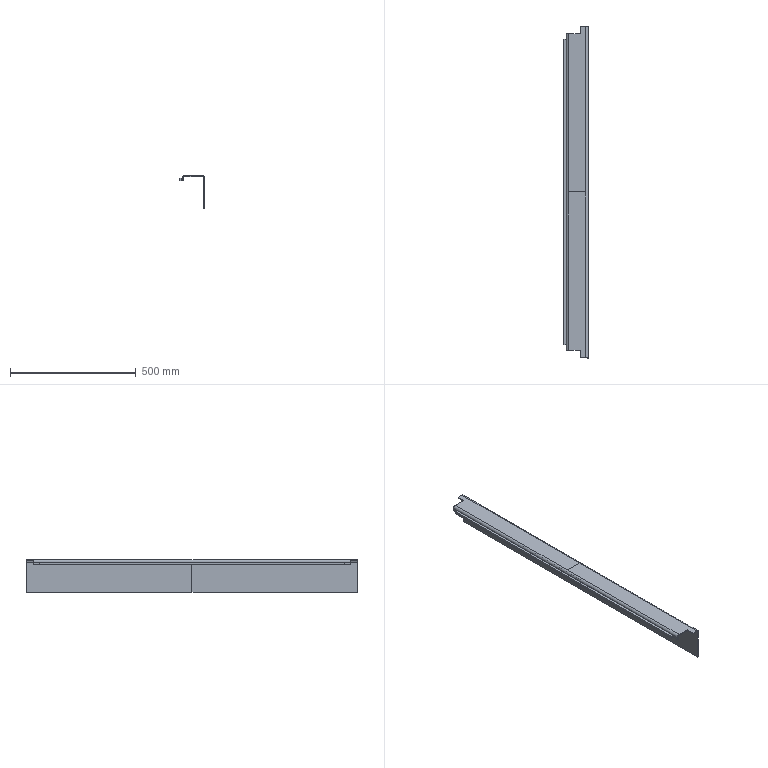Part | NX | features BREP 2 | 2 solids | 32 faces | box 98.003 x 1318 x 131 mm | volume 1286068 mm3 | plane 26 | cylinder 6 | commonest cylinder face diameters 12 x4 20 x2
STEP:
#1=CARTESIAN_POINT('',(588.385,607.17,426.));
#2=VERTEX_POINT('',#1);
#3=CARTESIAN_POINT('',(588.385,607.17,416.));
#4=VERTEX_POINT('',#3);
#5=CARTESIAN_POINT('',(588.385,607.17,421.));
#6=DIRECTION('',(0.000000043,0.,-1.));
#7=VECTOR('',#6,1000.);
#8=LINE('',#5,#7);
#9=EDGE_CURVE('',#2,#4,#8,.T.);
#10=ORIENTED_EDGE('',*,*,#9,.T.);
#11=CARTESIAN_POINT('',(582.385,607.17,416.));
#12=VERTEX_POINT('',#11);
#13=CARTESIAN_POINT('',(585.385,607.17,416.));
#14=DIRECTION('',(-1.,0.,0.));
#15=VECTOR('',#14,1000.);
#16=LINE('',#13,#15);
#17=EDGE_CURVE('',#4,#12,#16,.T.);
#18=ORIENTED_EDGE('',*,*,#17,.T.);
#19=CARTESIAN_POINT('',(582.385,607.17,426.));
#20=VERTEX_POINT('',#19);
#21=CARTESIAN_POINT('',(582.385,607.17,421.));
#22=DIRECTION('',(0.,0.,-1.));
#23=VECTOR('',#22,1000.);
#24=LINE('',#21,#23);
#25=EDGE_CURVE('',#20,#12,#24,.T.);
#26=ORIENTED_EDGE('',*,*,#25,.F.);
#27=CARTESIAN_POINT('',(585.385,607.17,426.));
#28=DIRECTION('',(-1.,0.,0.));
#29=VECTOR('',#28,1000.);
#30=LINE('',#27,#29);
#31=EDGE_CURVE('',#2,#20,#30,.T.);
#32=ORIENTED_EDGE('',*,*,#31,.F.);
#33=EDGE_LOOP('',(#10,#18,#26,#32));
#34=FACE_BOUND('',#33,.T.);
#35=CARTESIAN_POINT('',(585.23,607.17,818.966));
#36=DIRECTION('',(0.,1.,0.));
#37=DIRECTION('',(0.,0.,1.));
#38=AXIS2_PLACEMENT_3D('',#35,#36,#37);
#39=PLANE('',#38);
#40=ADVANCED_FACE('',(#34),#39,.T.);
#41=CARTESIAN_POINT('',(592.385,607.17,426.));
#42=VERTEX_POINT('',#41);
#43=CARTESIAN_POINT('',(592.385,607.17,416.));
#44=VERTEX_POINT('',#43);
#45=CARTESIAN_POINT('',(592.385,607.17,421.));
#46=DIRECTION('',(0.,0.,-1.));
#47=VECTOR('',#46,1000.);
#48=LINE('',#45,#47);
#49=EDGE_CURVE('',#42,#44,#48,.T.);
#50=ORIENTED_EDGE('',*,*,#49,.T.);
#51=CARTESIAN_POINT('',(590.385,607.17,416.));
#52=DIRECTION('',(-1.,0.,0.));
#53=VECTOR('',#52,1000.);
#54=LINE('',#51,#53);
#55=EDGE_CURVE('',#44,#4,#54,.T.);
#56=ORIENTED_EDGE('',*,*,#55,.T.);
#57=ORIENTED_EDGE('',*,*,#9,.F.);
#58=CARTESIAN_POINT('',(590.385,607.17,426.));
#59=DIRECTION('',(-1.,0.,0.));
#60=VECTOR('',#59,1000.);
#61=LINE('',#58,#60);
#62=EDGE_CURVE('',#42,#2,#61,.T.);
#63=ORIENTED_EDGE('',*,*,#62,.F.);
#64=EDGE_LOOP('',(#50,#56,#57,#63));
#65=FACE_BOUND('',#64,.T.);
#66=CARTESIAN_POINT('',(590.385,607.17,401.771));
#67=DIRECTION('',(0.,-1.,0.));
#68=DIRECTION('',(1.,0.,0.000000043));
#69=AXIS2_PLACEMENT_3D('',#66,#67,#68);
#70=PLANE('',#69);
#71=ADVANCED_FACE('',(#65),#70,.F.);
#72=ORIENTED_EDGE('',*,*,#49,.F.);
#73=CARTESIAN_POINT('',(592.385,-607.17,426.));
#74=VERTEX_POINT('',#73);
#75=CARTESIAN_POINT('',(592.385,0.,426.));
#76=DIRECTION('',(0.,1.,0.));
#77=VECTOR('',#76,1000.);
#78=LINE('',#75,#77);
#79=EDGE_CURVE('',#74,#42,#78,.T.);
#80=ORIENTED_EDGE('',*,*,#79,.F.);
#81=CARTESIAN_POINT('',(592.385,-607.17,416.));
#82=VERTEX_POINT('',#81);
#83=CARTESIAN_POINT('',(592.385,-607.17,421.));
#84=DIRECTION('',(0.,0.,1.));
#85=VECTOR('',#84,1000.);
#86=LINE('',#83,#85);
#87=EDGE_CURVE('',#82,#74,#86,.T.);
#88=ORIENTED_EDGE('',*,*,#87,.F.);
#89=CARTESIAN_POINT('',(592.385,0.,416.));
#90=DIRECTION('',(0.,1.,0.));
#91=VECTOR('',#90,1000.);
#92=LINE('',#89,#91);
#93=EDGE_CURVE('',#82,#44,#92,.T.);
#94=ORIENTED_EDGE('',*,*,#93,.T.);
#95=EDGE_LOOP('',(#72,#80,#88,#94));
#96=FACE_BOUND('',#95,.T.);
#97=CARTESIAN_POINT('',(592.385,0.,426.));
#98=DIRECTION('',(-1.,0.,0.));
#99=DIRECTION('',(0.,0.,-1.));
#100=AXIS2_PLACEMENT_3D('',#97,#98,#99);
#101=PLANE('',#100);
#102=ADVANCED_FACE('',(#96),#101,.F.);
#103=CARTESIAN_POINT('',(588.385,-607.17,426.));
#104=VERTEX_POINT('',#103);
#105=CARTESIAN_POINT('',(590.385,-607.17,426.));
#106=DIRECTION('',(-1.,0.,0.));
#107=VECTOR('',#106,1000.);
#108=LINE('',#105,#107);
#109=EDGE_CURVE('',#74,#104,#108,.T.);
#110=ORIENTED_EDGE('',*,*,#109,.T.);
#111=CARTESIAN_POINT('',(588.385,-607.17,416.));
#112=VERTEX_POINT('',#111);
#113=CARTESIAN_POINT('',(588.385,-607.17,426.));
#114=CARTESIAN_POINT('',(588.385,-607.17,424.));
#115=CARTESIAN_POINT('',(588.385,-607.17,422.));
#116=CARTESIAN_POINT('',(588.385,-607.17,420.));
#117=CARTESIAN_POINT('',(588.385,-607.17,418.));
#118=CARTESIAN_POINT('',(588.385,-607.17,416.));
#119=B_SPLINE_CURVE_WITH_KNOTS('',5,(#113,#114,#115,#116,#117,#118),.UNSPECIFIED.,.F.,.F.,(6,6),(830.931,840.931),.UNSPECIFIED.);
#120=EDGE_CURVE('',#104,#112,#119,.T.);
#121=ORIENTED_EDGE('',*,*,#120,.T.);
#122=CARTESIAN_POINT('',(590.385,-607.17,416.));
#123=DIRECTION('',(-1.,0.,0.));
#124=VECTOR('',#123,1000.);
#125=LINE('',#122,#124);
#126=EDGE_CURVE('',#82,#112,#125,.T.);
#127=ORIENTED_EDGE('',*,*,#126,.F.);
#128=ORIENTED_EDGE('',*,*,#87,.T.);
#129=EDGE_LOOP('',(#110,#121,#127,#128));
#130=FACE_BOUND('',#129,.T.);
#131=CARTESIAN_POINT('',(590.385,-607.17,401.771));
#132=DIRECTION('',(0.,-1.,0.));
#133=DIRECTION('',(1.,0.,0.000000043));
#134=AXIS2_PLACEMENT_3D('',#131,#132,#133);
#135=PLANE('',#134);
#136=ADVANCED_FACE('',(#130),#135,.T.);
#137=ORIENTED_EDGE('',*,*,#93,.F.);
#138=ORIENTED_EDGE('',*,*,#126,.T.);
#139=CARTESIAN_POINT('',(582.385,-607.17,416.));
#140=VERTEX_POINT('',#139);
#141=CARTESIAN_POINT('',(588.385,-607.17,416.));
#142=CARTESIAN_POINT('',(582.385,-607.17,416.));
#143=B_SPLINE_CURVE_WITH_KNOTS('',1,(#141,#142),.UNSPECIFIED.,.F.,.F.,(2,2),(0.,6.),.UNSPECIFIED.);
#144=EDGE_CURVE('',#112,#140,#143,.T.);
#145=ORIENTED_EDGE('',*,*,#144,.T.);
#146=CARTESIAN_POINT('',(582.385,0.,416.));
#147=DIRECTION('',(0.,1.,0.));
#148=VECTOR('',#147,1000.);
#149=LINE('',#146,#148);
#150=EDGE_CURVE('',#140,#12,#149,.T.);
#151=ORIENTED_EDGE('',*,*,#150,.T.);
#152=ORIENTED_EDGE('',*,*,#17,.F.);
#153=ORIENTED_EDGE('',*,*,#55,.F.);
#154=EDGE_LOOP('',(#137,#138,#145,#151,#152,#153));
#155=FACE_BOUND('',#154,.T.);
#156=CARTESIAN_POINT('',(582.385,0.,416.));
#157=DIRECTION('',(0.,0.,-1.));
#158=DIRECTION('',(1.,0.,0.));
#159=AXIS2_PLACEMENT_3D('',#156,#157,#158);
#160=PLANE('',#159);
#161=ADVANCED_FACE('',(#155),#160,.T.);
#162=ORIENTED_EDGE('',*,*,#25,.T.);
#163=ORIENTED_EDGE('',*,*,#150,.F.);
#164=CARTESIAN_POINT('',(582.385,-607.17,426.));
#165=VERTEX_POINT('',#164);
#166=CARTESIAN_POINT('',(582.385,-607.17,426.));
#167=CARTESIAN_POINT('',(582.385,-607.17,424.));
#168=CARTESIAN_POINT('',(582.385,-607.17,422.));
#169=CARTESIAN_POINT('',(582.385,-607.17,420.));
#170=CARTESIAN_POINT('',(582.385,-607.17,418.));
#171=CARTESIAN_POINT('',(582.385,-607.17,416.));
#172=B_SPLINE_CURVE_WITH_KNOTS('',5,(#166,#167,#168,#169,#170,#171),.UNSPECIFIED.,.F.,.F.,(6,6),(830.931,840.931),.UNSPECIFIED.);
#173=EDGE_CURVE('',#165,#140,#172,.T.);
#174=ORIENTED_EDGE('',*,*,#173,.F.);
#175=CARTESIAN_POINT('',(582.385,0.,426.));
#176=DIRECTION('',(0.,1.,0.));
#177=VECTOR('',#176,1000.);
#178=LINE('',#175,#177);
#179=EDGE_CURVE('',#165,#20,#178,.T.);
#180=ORIENTED_EDGE('',*,*,#179,.T.);
#181=EDGE_LOOP('',(#162,#163,#174,#180));
#182=FACE_BOUND('',#181,.T.);
#183=CARTESIAN_POINT('',(582.385,0.,416.));
#184=DIRECTION('',(1.,0.,0.));
#185=DIRECTION('',(0.,0.,1.));
#186=AXIS2_PLACEMENT_3D('',#183,#184,#185);
#187=PLANE('',#186);
#188=ADVANCED_FACE('',(#182),#187,.F.);
#189=ORIENTED_EDGE('',*,*,#179,.F.);
#190=CARTESIAN_POINT('',(588.385,-607.17,426.));
#191=CARTESIAN_POINT('',(582.385,-607.17,426.));
#192=B_SPLINE_CURVE_WITH_KNOTS('',1,(#190,#191),.UNSPECIFIED.,.F.,.F.,(2,2),(0.,6.),.UNSPECIFIED.);
#193=EDGE_CURVE('',#104,#165,#192,.T.);
#194=ORIENTED_EDGE('',*,*,#193,.F.);
#195=ORIENTED_EDGE('',*,*,#109,.F.);
#196=ORIENTED_EDGE('',*,*,#79,.T.);
#197=ORIENTED_EDGE('',*,*,#62,.T.);
#198=ORIENTED_EDGE('',*,*,#31,.T.);
#199=EDGE_LOOP('',(#189,#194,#195,#196,#197,#198));
#200=FACE_BOUND('',#199,.T.);
#201=CARTESIAN_POINT('',(592.385,0.,426.));
#202=DIRECTION('',(0.,0.,1.));
#203=DIRECTION('',(-1.,0.,0.));
#204=AXIS2_PLACEMENT_3D('',#201,#202,#203);
#205=PLANE('',#204);
#206=ADVANCED_FACE('',(#200),#205,.T.);
#207=ORIENTED_EDGE('',*,*,#193,.T.);
#208=ORIENTED_EDGE('',*,*,#173,.T.);
#209=ORIENTED_EDGE('',*,*,#144,.F.);
#210=ORIENTED_EDGE('',*,*,#120,.F.);
#211=EDGE_LOOP('',(#207,#208,#209,#210));
#212=FACE_BOUND('',#211,.T.);
#213=CARTESIAN_POINT('',(585.23,-607.17,818.966));
#214=DIRECTION('',(0.,1.,0.));
#215=DIRECTION('',(0.,0.,1.));
#216=AXIS2_PLACEMENT_3D('',#213,#214,#215);
#217=PLANE('',#216);
#218=ADVANCED_FACE('',(#212),#217,.F.);
#219=CLOSED_SHELL('',(#40,#71,#102,#136,#161,#188,#206,#218));
#220=MANIFOLD_SOLID_BREP('',#219);
#221=CARTESIAN_POINT('',(592.385,-628.17,416.));
#222=VERTEX_POINT('',#221);
#223=CARTESIAN_POINT('',(592.385,628.17,416.));
#224=VERTEX_POINT('',#223);
#225=CARTESIAN_POINT('',(592.385,0.,416.));
#226=DIRECTION('',(0.,1.,0.));
#227=VECTOR('',#226,1000.);
#228=LINE('',#225,#227);
#229=EDGE_CURVE('',#222,#224,#228,.T.);
#230=ORIENTED_EDGE('',*,*,#229,.F.);
#231=CARTESIAN_POINT('',(592.385,-628.17,426.));
#232=VERTEX_POINT('',#231);
#233=CARTESIAN_POINT('',(592.385,-628.17,421.));
#234=DIRECTION('',(0.,0.,1.));
#235=VECTOR('',#234,1000.);
#236=LINE('',#233,#235);
#237=EDGE_CURVE('',#222,#232,#236,.T.);
#238=ORIENTED_EDGE('',*,*,#237,.T.);
#239=CARTESIAN_POINT('',(592.385,628.17,426.));
#240=VERTEX_POINT('',#239);
#241=CARTESIAN_POINT('',(592.385,-322.5,426.));
#242=DIRECTION('',(0.,-1.,0.));
#243=VECTOR('',#242,1000.);
#244=LINE('',#241,#243);
#245=EDGE_CURVE('',#240,#232,#244,.T.);
#246=ORIENTED_EDGE('',*,*,#245,.F.);
#247=CARTESIAN_POINT('',(592.385,628.17,421.));
#248=DIRECTION('',(0.,0.,1.));
#249=VECTOR('',#248,1000.);
#250=LINE('',#247,#249);
#251=EDGE_CURVE('',#224,#240,#250,.T.);
#252=ORIENTED_EDGE('',*,*,#251,.F.);
#253=EDGE_LOOP('',(#230,#238,#246,#252));
#254=FACE_BOUND('',#253,.T.);
#255=CARTESIAN_POINT('',(592.385,0.,436.));
#256=DIRECTION('',(-1.,0.,0.));
#257=DIRECTION('',(0.,-1.,0.));
#258=AXIS2_PLACEMENT_3D('',#255,#256,#257);
#259=PLANE('',#258);
#260=ADVANCED_FACE('',(#254),#259,.T.);
#261=CARTESIAN_POINT('',(596.385,628.17,416.));
#262=VERTEX_POINT('',#261);
#263=CARTESIAN_POINT('',(594.385,628.17,416.));
#264=DIRECTION('',(1.,0.,0.));
#265=VECTOR('',#264,1000.);
#266=LINE('',#263,#265);
#267=EDGE_CURVE('',#224,#262,#266,.T.);
#268=ORIENTED_EDGE('',*,*,#267,.T.);
#269=CARTESIAN_POINT('',(596.385,-628.17,416.));
#270=VERTEX_POINT('',#269);
#271=CARTESIAN_POINT('',(596.385,0.,416.));
#272=DIRECTION('',(0.,-1.,0.));
#273=VECTOR('',#272,1000.);
#274=LINE('',#271,#273);
#275=EDGE_CURVE('',#262,#270,#274,.T.);
#276=ORIENTED_EDGE('',*,*,#275,.T.);
#277=CARTESIAN_POINT('',(594.385,-628.17,416.));
#278=DIRECTION('',(1.,0.,0.));
#279=VECTOR('',#278,1000.);
#280=LINE('',#277,#279);
#281=EDGE_CURVE('',#222,#270,#280,.T.);
#282=ORIENTED_EDGE('',*,*,#281,.F.);
#283=ORIENTED_EDGE('',*,*,#229,.T.);
#284=EDGE_LOOP('',(#268,#276,#282,#283));
#285=FACE_BOUND('',#284,.T.);
#286=CARTESIAN_POINT('',(592.385,-322.5,416.));
#287=DIRECTION('',(0.,0.,1.));
#288=DIRECTION('',(1.,0.,0.));
#289=AXIS2_PLACEMENT_3D('',#286,#287,#288);
#290=PLANE('',#289);
#291=ADVANCED_FACE('',(#285),#290,.F.);
#292=CARTESIAN_POINT('',(596.385,628.17,426.));
#293=VERTEX_POINT('',#292);
#294=CARTESIAN_POINT('',(596.385,628.17,421.));
#295=DIRECTION('',(0.,0.,1.));
#296=VECTOR('',#295,1000.);
#297=LINE('',#294,#296);
#298=EDGE_CURVE('',#262,#293,#297,.T.);
#299=ORIENTED_EDGE('',*,*,#298,.T.);
#300=CARTESIAN_POINT('',(596.385,-628.17,426.));
#301=VERTEX_POINT('',#300);
#302=CARTESIAN_POINT('',(596.385,-322.5,426.));
#303=DIRECTION('',(0.,-1.,0.));
#304=VECTOR('',#303,1000.);
#305=LINE('',#302,#304);
#306=EDGE_CURVE('',#293,#301,#305,.T.);
#307=ORIENTED_EDGE('',*,*,#306,.T.);
#308=CARTESIAN_POINT('',(596.385,-628.17,421.));
#309=DIRECTION('',(0.,0.,1.));
#310=VECTOR('',#309,1000.);
#311=LINE('',#308,#310);
#312=EDGE_CURVE('',#270,#301,#311,.T.);
#313=ORIENTED_EDGE('',*,*,#312,.F.);
#314=ORIENTED_EDGE('',*,*,#275,.F.);
#315=EDGE_LOOP('',(#299,#307,#313,#314));
#316=FACE_BOUND('',#315,.T.);
#317=CARTESIAN_POINT('',(596.385,0.,436.));
#318=DIRECTION('',(-1.,0.,0.));
#319=DIRECTION('',(0.,-1.,0.));
#320=AXIS2_PLACEMENT_3D('',#317,#318,#319);
#321=PLANE('',#320);
#322=ADVANCED_FACE('',(#316),#321,.F.);
#323=CARTESIAN_POINT('',(598.143,-628.17,430.243));
#324=VERTEX_POINT('',#323);
#325=CARTESIAN_POINT('',(596.385,-628.17,426.));
#326=CARTESIAN_POINT('',(596.385,-628.17,427.576));
#327=CARTESIAN_POINT('',(597.028,-628.17,429.128));
#328=CARTESIAN_POINT('',(598.143,-628.17,430.243));
#329=B_SPLINE_CURVE_WITH_KNOTS('',3,(#325,#326,#327,#328),.UNSPECIFIED.,.F.,.F.,(4,4),(0.,1.),.UNSPECIFIED.);
#330=EDGE_CURVE('',#301,#324,#329,.T.);
#331=ORIENTED_EDGE('',*,*,#330,.F.);
#332=ORIENTED_EDGE('',*,*,#306,.F.);
#333=CARTESIAN_POINT('',(598.143,628.17,430.243));
#334=VERTEX_POINT('',#333);
#335=CARTESIAN_POINT('',(598.143,628.17,430.243));
#336=CARTESIAN_POINT('',(597.96,628.17,430.061));
#337=CARTESIAN_POINT('',(597.788,628.17,429.869));
#338=CARTESIAN_POINT('',(597.626,628.17,429.668));
#339=CARTESIAN_POINT('',(597.124,628.17,428.971));
#340=CARTESIAN_POINT('',(596.751,628.17,428.192));
#341=CARTESIAN_POINT('',(596.56,628.17,427.616));
#342=CARTESIAN_POINT('',(596.426,628.17,426.939));
#343=CARTESIAN_POINT('',(596.39,628.17,426.255));
#344=CARTESIAN_POINT('',(596.387,628.17,426.17));
#345=CARTESIAN_POINT('',(596.385,628.17,426.085));
#346=CARTESIAN_POINT('',(596.385,628.17,426.));
#347=B_SPLINE_CURVE_WITH_KNOTS('',5,(#335,#336,#337,#338,#339,#340,#341,#342,#343,#344,#345,#346),.UNSPECIFIED.,.F.,.F.,(6,3,3,6),(6.664,8.485,12.728,13.328),.UNSPECIFIED.);
#348=EDGE_CURVE('',#334,#293,#347,.T.);
#349=ORIENTED_EDGE('',*,*,#348,.F.);
#350=CARTESIAN_POINT('',(598.143,-322.5,430.243));
#351=DIRECTION('',(0.,-1.,0.));
#352=VECTOR('',#351,1000.);
#353=LINE('',#350,#352);
#354=EDGE_CURVE('',#334,#324,#353,.T.);
#355=ORIENTED_EDGE('',*,*,#354,.T.);
#356=EDGE_LOOP('',(#331,#332,#349,#355));
#357=FACE_BOUND('',#356,.T.);
#358=CARTESIAN_POINT('',(602.385,-322.5,426.));
#359=DIRECTION('',(0.,-1.,0.));
#360=DIRECTION('',(-0.7071,0.,0.7071));
#361=AXIS2_PLACEMENT_3D('',#358,#359,#360);
#362=CYLINDRICAL_SURFACE('',#361,6.);
#363=ADVANCED_FACE('',(#357),#362,.F.);
#364=ORIENTED_EDGE('',*,*,#312,.T.);
#365=ORIENTED_EDGE('',*,*,#330,.T.);
#366=CARTESIAN_POINT('',(602.385,-628.17,432.));
#367=VERTEX_POINT('',#366);
#368=CARTESIAN_POINT('',(598.143,-628.17,430.243));
#369=CARTESIAN_POINT('',(599.256,-628.17,431.357));
#370=CARTESIAN_POINT('',(600.809,-628.17,432.));
#371=CARTESIAN_POINT('',(602.385,-628.17,432.));
#372=B_SPLINE_CURVE_WITH_KNOTS('',3,(#368,#369,#370,#371),.UNSPECIFIED.,.F.,.F.,(4,4),(0.,1.),.UNSPECIFIED.);
#373=EDGE_CURVE('',#324,#367,#372,.T.);
#374=ORIENTED_EDGE('',*,*,#373,.T.);
#375=CARTESIAN_POINT('',(648.674,-628.17,432.));
#376=VERTEX_POINT('',#375);
#377=CARTESIAN_POINT('',(625.529,-628.17,432.));
#378=DIRECTION('',(-1.,0.,0.));
#379=VECTOR('',#378,1000.);
#380=LINE('',#377,#379);
#381=EDGE_CURVE('',#376,#367,#380,.T.);
#382=ORIENTED_EDGE('',*,*,#381,.F.);
#383=CARTESIAN_POINT('',(648.674,-628.17,436.));
#384=VERTEX_POINT('',#383);
#385=CARTESIAN_POINT('',(648.674,-628.17,434.));
#386=DIRECTION('',(0.,0.,-1.));
#387=VECTOR('',#386,1000.);
#388=LINE('',#385,#387);
#389=EDGE_CURVE('',#384,#376,#388,.T.);
#390=ORIENTED_EDGE('',*,*,#389,.F.);
#391=CARTESIAN_POINT('',(602.385,-628.17,436.));
#392=VERTEX_POINT('',#391);
#393=CARTESIAN_POINT('',(625.529,-628.17,436.));
#394=DIRECTION('',(-1.,0.,0.));
#395=VECTOR('',#394,1000.);
#396=LINE('',#393,#395);
#397=EDGE_CURVE('',#384,#392,#396,.T.);
#398=ORIENTED_EDGE('',*,*,#397,.T.);
#399=CARTESIAN_POINT('',(602.385,-628.17,426.));
#400=DIRECTION('',(0.,-1.,0.));
#401=DIRECTION('',(1.,0.,0.));
#402=AXIS2_PLACEMENT_3D('',#399,#400,#401);
#403=CIRCLE('',#402,10.);
#404=EDGE_CURVE('',#392,#232,#403,.T.);
#405=ORIENTED_EDGE('',*,*,#404,.T.);
#406=ORIENTED_EDGE('',*,*,#237,.F.);
#407=ORIENTED_EDGE('',*,*,#281,.T.);
#408=EDGE_LOOP('',(#364,#365,#374,#382,#390,#398,#405,#406,#407));
#409=FACE_BOUND('',#408,.T.);
#410=CARTESIAN_POINT('',(578.388,-628.17,381.004));
#411=DIRECTION('',(0.,1.,0.));
#412=DIRECTION('',(0.,0.,1.));
#413=AXIS2_PLACEMENT_3D('',#410,#411,#412);
#414=PLANE('',#413);
#415=ADVANCED_FACE('',(#409),#414,.F.);
#416=CARTESIAN_POINT('',(602.385,628.17,432.));
#417=VERTEX_POINT('',#416);
#418=CARTESIAN_POINT('',(602.385,628.17,432.));
#419=CARTESIAN_POINT('',(601.785,628.17,432.));
#420=CARTESIAN_POINT('',(601.185,628.17,431.925));
#421=CARTESIAN_POINT('',(600.598,628.17,431.775));
#422=CARTESIAN_POINT('',(599.714,628.17,431.427));
#423=CARTESIAN_POINT('',(598.919,628.17,430.916));
#424=CARTESIAN_POINT('',(598.644,628.17,430.71));
#425=CARTESIAN_POINT('',(598.385,628.17,430.485));
#426=CARTESIAN_POINT('',(598.143,628.17,430.243));
#427=B_SPLINE_CURVE_WITH_KNOTS('',5,(#418,#419,#420,#421,#422,#423,#424,#425,#426),.UNSPECIFIED.,.F.,.F.,(6,3,6),(0.,4.243,6.664),.UNSPECIFIED.);
#428=EDGE_CURVE('',#417,#334,#427,.T.);
#429=ORIENTED_EDGE('',*,*,#428,.F.);
#430=CARTESIAN_POINT('',(602.385,0.,432.));
#431=VERTEX_POINT('',#430);
#432=CARTESIAN_POINT('',(602.385,314.085,432.));
#433=DIRECTION('',(0.,-1.,0.));
#434=VECTOR('',#433,1000.);
#435=LINE('',#432,#434);
#436=EDGE_CURVE('',#417,#431,#435,.T.);
#437=ORIENTED_EDGE('',*,*,#436,.T.);
#438=CARTESIAN_POINT('',(602.385,-314.085,432.));
#439=DIRECTION('',(0.,-1.,0.));
#440=VECTOR('',#439,1000.);
#441=LINE('',#438,#440);
#442=EDGE_CURVE('',#431,#367,#441,.T.);
#443=ORIENTED_EDGE('',*,*,#442,.T.);
#444=ORIENTED_EDGE('',*,*,#373,.F.);
#445=ORIENTED_EDGE('',*,*,#354,.F.);
#446=EDGE_LOOP('',(#429,#437,#443,#444,#445));
#447=FACE_BOUND('',#446,.T.);
#448=CARTESIAN_POINT('',(602.385,-322.5,426.));
#449=DIRECTION('',(0.,-1.,0.));
#450=DIRECTION('',(0.7071,0.,-0.7071));
#451=AXIS2_PLACEMENT_3D('',#448,#449,#450);
#452=CYLINDRICAL_SURFACE('',#451,6.);
#453=ADVANCED_FACE('',(#447),#452,.F.);
#454=CARTESIAN_POINT('',(602.385,628.17,436.));
#455=VERTEX_POINT('',#454);
#456=CARTESIAN_POINT('',(602.385,0.,436.));
#457=VERTEX_POINT('',#456);
#458=CARTESIAN_POINT('',(602.385,314.085,436.));
#459=DIRECTION('',(0.,-1.,0.));
#460=VECTOR('',#459,1000.);
#461=LINE('',#458,#460);
#462=EDGE_CURVE('',#455,#457,#461,.T.);
#463=ORIENTED_EDGE('',*,*,#462,.F.);
#464=CARTESIAN_POINT('',(592.385,628.17,426.));
#465=CARTESIAN_POINT('',(592.385,628.17,428.627));
#466=CARTESIAN_POINT('',(594.557,628.17,433.83));
#467=CARTESIAN_POINT('',(599.758,628.17,436.));
#468=CARTESIAN_POINT('',(602.385,628.17,436.));
#469=B_SPLINE_CURVE_WITH_KNOTS('',3,(#464,#465,#466,#467,#468),.UNSPECIFIED.,.F.,.F.,(4,1,4),(0.,0.5,1.),.UNSPECIFIED.);
#470=EDGE_CURVE('',#455,#240,#469,.F.);
#471=ORIENTED_EDGE('',*,*,#470,.T.);
#472=ORIENTED_EDGE('',*,*,#245,.T.);
#473=ORIENTED_EDGE('',*,*,#404,.F.);
#474=CARTESIAN_POINT('',(602.385,-314.085,436.));
#475=DIRECTION('',(0.,-1.,0.));
#476=VECTOR('',#475,1000.);
#477=LINE('',#474,#476);
#478=EDGE_CURVE('',#457,#392,#477,.T.);
#479=ORIENTED_EDGE('',*,*,#478,.F.);
#480=EDGE_LOOP('',(#463,#471,#472,#473,#479));
#481=FACE_BOUND('',#480,.T.);
#482=CARTESIAN_POINT('',(602.385,-322.5,426.));
#483=DIRECTION('',(0.,-1.,0.));
#484=DIRECTION('',(0.,0.,1.));
#485=AXIS2_PLACEMENT_3D('',#482,#483,#484);
#486=CYLINDRICAL_SURFACE('',#485,10.);
#487=ADVANCED_FACE('',(#481),#486,.T.);
#488=CARTESIAN_POINT('',(648.674,628.17,432.));
#489=VERTEX_POINT('',#488);
#490=CARTESIAN_POINT('',(625.529,628.17,432.));
#491=DIRECTION('',(-1.,0.,0.));
#492=VECTOR('',#491,1000.);
#493=LINE('',#490,#492);
#494=EDGE_CURVE('',#489,#417,#493,.T.);
#495=ORIENTED_EDGE('',*,*,#494,.T.);
#496=ORIENTED_EDGE('',*,*,#428,.T.);
#497=ORIENTED_EDGE('',*,*,#348,.T.);
#498=ORIENTED_EDGE('',*,*,#298,.F.);
#499=ORIENTED_EDGE('',*,*,#267,.F.);
#500=ORIENTED_EDGE('',*,*,#251,.T.);
#501=ORIENTED_EDGE('',*,*,#470,.F.);
#502=CARTESIAN_POINT('',(648.674,628.17,436.));
#503=VERTEX_POINT('',#502);
#504=CARTESIAN_POINT('',(625.529,628.17,436.));
#505=DIRECTION('',(-1.,0.,0.));
#506=VECTOR('',#505,1000.);
#507=LINE('',#504,#506);
#508=EDGE_CURVE('',#503,#455,#507,.T.);
#509=ORIENTED_EDGE('',*,*,#508,.F.);
#510=CARTESIAN_POINT('',(648.674,628.17,434.));
#511=DIRECTION('',(0.,0.,-1.));
#512=VECTOR('',#511,1000.);
#513=LINE('',#510,#512);
#514=EDGE_CURVE('',#503,#489,#513,.T.);
#515=ORIENTED_EDGE('',*,*,#514,.T.);
#516=EDGE_LOOP('',(#495,#496,#497,#498,#499,#500,#501,#509,#515));
#517=FACE_BOUND('',#516,.T.);
#518=CARTESIAN_POINT('',(578.388,628.17,381.004));
#519=DIRECTION('',(0.,1.,0.));
#520=DIRECTION('',(0.,0.,1.));
#521=AXIS2_PLACEMENT_3D('',#518,#519,#520);
#522=PLANE('',#521);
#523=ADVANCED_FACE('',(#517),#522,.T.);
#524=ORIENTED_EDGE('',*,*,#442,.F.);
#525=CARTESIAN_POINT('',(670.388,0.,432.));
#526=VERTEX_POINT('',#525);
#527=CARTESIAN_POINT('',(636.387,-0.000000001,432.));
#528=DIRECTION('',(-1.,0.,0.));
#529=VECTOR('',#528,1000.);
#530=LINE('',#527,#529);
#531=EDGE_CURVE('',#526,#431,#530,.T.);
#532=ORIENTED_EDGE('',*,*,#531,.F.);
#533=CARTESIAN_POINT('',(670.388,-659.,432.));
#534=VERTEX_POINT('',#533);
#535=CARTESIAN_POINT('',(670.388,-322.5,432.));
#536=DIRECTION('',(0.,1.,0.));
#537=VECTOR('',#536,1000.);
#538=LINE('',#535,#537);
#539=EDGE_CURVE('',#534,#526,#538,.T.);
#540=ORIENTED_EDGE('',*,*,#539,.F.);
#541=CARTESIAN_POINT('',(648.674,-659.,432.));
#542=VERTEX_POINT('',#541);
#543=CARTESIAN_POINT('',(659.531,-659.,432.));
#544=DIRECTION('',(-1.,0.,0.));
#545=VECTOR('',#544,1000.);
#546=LINE('',#543,#545);
#547=EDGE_CURVE('',#534,#542,#546,.T.);
#548=ORIENTED_EDGE('',*,*,#547,.T.);
#549=CARTESIAN_POINT('',(648.674,-643.585,432.));
#550=DIRECTION('',(0.,1.,0.));
#551=VECTOR('',#550,1000.);
#552=LINE('',#549,#551);
#553=EDGE_CURVE('',#542,#376,#552,.T.);
#554=ORIENTED_EDGE('',*,*,#553,.T.);
#555=ORIENTED_EDGE('',*,*,#381,.T.);
#556=EDGE_LOOP('',(#524,#532,#540,#548,#554,#555));
#557=FACE_BOUND('',#556,.T.);
#558=CARTESIAN_POINT('',(670.388,0.,432.));
#559=DIRECTION('',(0.,0.,-1.));
#560=DIRECTION('',(0.,-1.,0.));
#561=AXIS2_PLACEMENT_3D('',#558,#559,#560);
#562=PLANE('',#561);
#563=ADVANCED_FACE('',(#557),#562,.T.);
#564=ORIENTED_EDGE('',*,*,#553,.F.);
#565=CARTESIAN_POINT('',(648.674,-659.,436.));
#566=VERTEX_POINT('',#565);
#567=CARTESIAN_POINT('',(648.674,-659.,434.));
#568=DIRECTION('',(0.,0.,1.));
#569=VECTOR('',#568,1000.);
#570=LINE('',#567,#569);
#571=EDGE_CURVE('',#542,#566,#570,.T.);
#572=ORIENTED_EDGE('',*,*,#571,.T.);
#573=CARTESIAN_POINT('',(648.674,-643.585,436.));
#574=DIRECTION('',(0.,1.,0.));
#575=VECTOR('',#574,1000.);
#576=LINE('',#573,#575);
#577=EDGE_CURVE('',#566,#384,#576,.T.);
#578=ORIENTED_EDGE('',*,*,#577,.T.);
#579=ORIENTED_EDGE('',*,*,#389,.T.);
#580=EDGE_LOOP('',(#564,#572,#578,#579));
#581=FACE_BOUND('',#580,.T.);
#582=CARTESIAN_POINT('',(648.674,-660.,1278.826));
#583=DIRECTION('',(1.,0.,0.));
#584=DIRECTION('',(0.,0.,-1.));
#585=AXIS2_PLACEMENT_3D('',#582,#583,#584);
#586=PLANE('',#585);
#587=ADVANCED_FACE('',(#581),#586,.F.);
#588=ORIENTED_EDGE('',*,*,#397,.F.);
#589=ORIENTED_EDGE('',*,*,#577,.F.);
#590=CARTESIAN_POINT('',(670.388,-659.,436.));
#591=VERTEX_POINT('',#590);
#592=CARTESIAN_POINT('',(659.531,-659.,436.));
#593=DIRECTION('',(-1.,0.,0.));
#594=VECTOR('',#593,1000.);
#595=LINE('',#592,#594);
#596=EDGE_CURVE('',#591,#566,#595,.T.);
#597=ORIENTED_EDGE('',*,*,#596,.F.);
#598=CARTESIAN_POINT('',(670.388,0.,436.));
#599=VERTEX_POINT('',#598);
#600=CARTESIAN_POINT('',(670.388,-322.5,436.));
#601=DIRECTION('',(0.,1.,0.));
#602=VECTOR('',#601,1000.);
#603=LINE('',#600,#602);
#604=EDGE_CURVE('',#591,#599,#603,.T.);
#605=ORIENTED_EDGE('',*,*,#604,.T.);
#606=CARTESIAN_POINT('',(636.387,-0.000000001,436.));
#607=DIRECTION('',(-1.,0.,0.));
#608=VECTOR('',#607,1000.);
#609=LINE('',#606,#608);
#610=EDGE_CURVE('',#599,#457,#609,.T.);
#611=ORIENTED_EDGE('',*,*,#610,.T.);
#612=ORIENTED_EDGE('',*,*,#478,.T.);
#613=EDGE_LOOP('',(#588,#589,#597,#605,#611,#612));
#614=FACE_BOUND('',#613,.T.);
#615=CARTESIAN_POINT('',(670.388,0.,436.));
#616=DIRECTION('',(0.,0.,-1.));
#617=DIRECTION('',(0.,-1.,0.));
#618=AXIS2_PLACEMENT_3D('',#615,#616,#617);
#619=PLANE('',#618);
#620=ADVANCED_FACE('',(#614),#619,.F.);
#621=CARTESIAN_POINT('',(648.674,659.,432.));
#622=VERTEX_POINT('',#621);
#623=CARTESIAN_POINT('',(648.674,643.585,432.));
#624=DIRECTION('',(0.,-1.,0.));
#625=VECTOR('',#624,1000.);
#626=LINE('',#623,#625);
#627=EDGE_CURVE('',#622,#489,#626,.T.);
#628=ORIENTED_EDGE('',*,*,#627,.T.);
#629=ORIENTED_EDGE('',*,*,#514,.F.);
#630=CARTESIAN_POINT('',(648.674,659.,436.));
#631=VERTEX_POINT('',#630);
#632=CARTESIAN_POINT('',(648.674,643.585,436.));
#633=DIRECTION('',(0.,-1.,0.));
#634=VECTOR('',#633,1000.);
#635=LINE('',#632,#634);
#636=EDGE_CURVE('',#631,#503,#635,.T.);
#637=ORIENTED_EDGE('',*,*,#636,.F.);
#638=CARTESIAN_POINT('',(648.674,659.,434.));
#639=DIRECTION('',(0.,0.,1.));
#640=VECTOR('',#639,1000.);
#641=LINE('',#638,#640);
#642=EDGE_CURVE('',#622,#631,#641,.T.);
#643=ORIENTED_EDGE('',*,*,#642,.F.);
#644=EDGE_LOOP('',(#628,#629,#637,#643));
#645=FACE_BOUND('',#644,.T.);
#646=CARTESIAN_POINT('',(648.674,660.,1278.826));
#647=DIRECTION('',(-1.,0.,0.));
#648=DIRECTION('',(0.,0.,-1.));
#649=AXIS2_PLACEMENT_3D('',#646,#647,#648);
#650=PLANE('',#649);
#651=ADVANCED_FACE('',(#645),#650,.T.);
#652=ORIENTED_EDGE('',*,*,#627,.F.);
#653=CARTESIAN_POINT('',(670.388,659.,432.));
#654=VERTEX_POINT('',#653);
#655=CARTESIAN_POINT('',(659.531,659.,432.));
#656=DIRECTION('',(-1.,0.,0.));
#657=VECTOR('',#656,1000.);
#658=LINE('',#655,#657);
#659=EDGE_CURVE('',#654,#622,#658,.T.);
#660=ORIENTED_EDGE('',*,*,#659,.F.);
#661=CARTESIAN_POINT('',(670.388,-322.5,432.));
#662=DIRECTION('',(0.,1.,0.));
#663=VECTOR('',#662,1000.);
#664=LINE('',#661,#663);
#665=EDGE_CURVE('',#526,#654,#664,.T.);
#666=ORIENTED_EDGE('',*,*,#665,.F.);
#667=ORIENTED_EDGE('',*,*,#531,.T.);
#668=ORIENTED_EDGE('',*,*,#436,.F.);
#669=ORIENTED_EDGE('',*,*,#494,.F.);
#670=EDGE_LOOP('',(#652,#660,#666,#667,#668,#669));
#671=FACE_BOUND('',#670,.T.);
#672=CARTESIAN_POINT('',(670.388,0.,432.));
#673=DIRECTION('',(0.,0.,1.));
#674=DIRECTION('',(0.,1.,0.));
#675=AXIS2_PLACEMENT_3D('',#672,#673,#674);
#676=PLANE('',#675);
#677=ADVANCED_FACE('',(#671),#676,.F.);
#678=CARTESIAN_POINT('',(674.631,-659.,430.243));
#679=VERTEX_POINT('',#678);
#680=CARTESIAN_POINT('',(670.388,-659.,432.));
#681=CARTESIAN_POINT('',(671.964,-659.,432.));
#682=CARTESIAN_POINT('',(673.516,-659.,431.358));
#683=CARTESIAN_POINT('',(674.631,-659.,430.243));
#684=B_SPLINE_CURVE_WITH_KNOTS('',3,(#680,#681,#682,#683),.UNSPECIFIED.,.F.,.F.,(4,4),(0.,1.),.UNSPECIFIED.);
#685=EDGE_CURVE('',#534,#679,#684,.T.);
#686=ORIENTED_EDGE('',*,*,#685,.F.);
#687=ORIENTED_EDGE('',*,*,#539,.T.);
#688=ORIENTED_EDGE('',*,*,#665,.T.);
#689=CARTESIAN_POINT('',(674.631,659.,430.243));
#690=VERTEX_POINT('',#689);
#691=CARTESIAN_POINT('',(670.388,659.,426.));
#692=DIRECTION('',(0.,1.,0.));
#693=DIRECTION('',(1.,0.,0.));
#694=AXIS2_PLACEMENT_3D('',#691,#692,#693);
#695=CIRCLE('',#694,6.);
#696=EDGE_CURVE('',#654,#690,#695,.T.);
#697=ORIENTED_EDGE('',*,*,#696,.T.);
#698=CARTESIAN_POINT('',(674.631,-322.5,430.243));
#699=DIRECTION('',(0.,1.,0.));
#700=VECTOR('',#699,1000.);
#701=LINE('',#698,#700);
#702=EDGE_CURVE('',#679,#690,#701,.T.);
#703=ORIENTED_EDGE('',*,*,#702,.F.);
#704=EDGE_LOOP('',(#686,#687,#688,#697,#703));
#705=FACE_BOUND('',#704,.T.);
#706=CARTESIAN_POINT('',(670.388,-322.5,426.));
#707=DIRECTION('',(0.,1.,0.));
#708=DIRECTION('',(-0.7071,0.,-0.7071));
#709=AXIS2_PLACEMENT_3D('',#706,#707,#708);
#710=CYLINDRICAL_SURFACE('',#709,6.);
#711=ADVANCED_FACE('',(#705),#710,.F.);
#712=CARTESIAN_POINT('',(680.388,0.,426.));
#713=VERTEX_POINT('',#712);
#714=CARTESIAN_POINT('',(680.388,659.,426.));
#715=VERTEX_POINT('',#714);
#716=CARTESIAN_POINT('',(680.388,329.5,426.));
#717=DIRECTION('',(0.,1.,0.));
#718=VECTOR('',#717,1000.);
#719=LINE('',#716,#718);
#720=EDGE_CURVE('',#713,#715,#719,.T.);
#721=ORIENTED_EDGE('',*,*,#720,.T.);
#722=CARTESIAN_POINT('',(670.388,659.,436.));
#723=VERTEX_POINT('',#722);
#724=CARTESIAN_POINT('',(670.388,659.,426.));
#725=DIRECTION('',(0.,1.,0.));
#726=DIRECTION('',(1.,0.,0.));
#727=AXIS2_PLACEMENT_3D('',#724,#725,#726);
#728=CIRCLE('',#727,10.);
#729=EDGE_CURVE('',#723,#715,#728,.T.);
#730=ORIENTED_EDGE('',*,*,#729,.F.);
#731=CARTESIAN_POINT('',(670.388,329.5,436.));
#732=DIRECTION('',(0.,1.,0.));
#733=VECTOR('',#732,1000.);
#734=LINE('',#731,#733);
#735=EDGE_CURVE('',#599,#723,#734,.T.);
#736=ORIENTED_EDGE('',*,*,#735,.F.);
#737=ORIENTED_EDGE('',*,*,#604,.F.);
#738=CARTESIAN_POINT('',(680.388,-659.,426.));
#739=VERTEX_POINT('',#738);
#740=CARTESIAN_POINT('',(680.388,-659.,426.));
#741=CARTESIAN_POINT('',(680.388,-659.,428.629));
#742=CARTESIAN_POINT('',(678.215,-659.,433.828));
#743=CARTESIAN_POINT('',(673.017,-659.,436.));
#744=CARTESIAN_POINT('',(670.388,-659.,436.));
#745=B_SPLINE_CURVE_WITH_KNOTS('',3,(#740,#741,#742,#743,#744),.UNSPECIFIED.,.F.,.F.,(4,1,4),(0.,0.5,1.),.UNSPECIFIED.);
#746=EDGE_CURVE('',#591,#739,#745,.F.);
#747=ORIENTED_EDGE('',*,*,#746,.T.);
#748=CARTESIAN_POINT('',(680.388,-329.5,426.));
#749=DIRECTION('',(0.,1.,0.));
#750=VECTOR('',#749,1000.);
#751=LINE('',#748,#750);
#752=EDGE_CURVE('',#739,#713,#751,.T.);
#753=ORIENTED_EDGE('',*,*,#752,.T.);
#754=EDGE_LOOP('',(#721,#730,#736,#737,#747,#753));
#755=FACE_BOUND('',#754,.T.);
#756=CARTESIAN_POINT('',(670.388,-322.5,426.));
#757=DIRECTION('',(0.,1.,0.));
#758=DIRECTION('',(0.,0.,1.));
#759=AXIS2_PLACEMENT_3D('',#756,#757,#758);
#760=CYLINDRICAL_SURFACE('',#759,10.);
#761=ADVANCED_FACE('',(#755),#760,.T.);
#762=ORIENTED_EDGE('',*,*,#636,.T.);
#763=ORIENTED_EDGE('',*,*,#508,.T.);
#764=ORIENTED_EDGE('',*,*,#462,.T.);
#765=ORIENTED_EDGE('',*,*,#610,.F.);
#766=ORIENTED_EDGE('',*,*,#735,.T.);
#767=CARTESIAN_POINT('',(659.531,659.,436.));
#768=DIRECTION('',(-1.,0.,0.));
#769=VECTOR('',#768,1000.);
#770=LINE('',#767,#769);
#771=EDGE_CURVE('',#723,#631,#770,.T.);
#772=ORIENTED_EDGE('',*,*,#771,.T.);
#773=EDGE_LOOP('',(#762,#763,#764,#765,#766,#772));
#774=FACE_BOUND('',#773,.T.);
#775=CARTESIAN_POINT('',(670.388,0.,436.));
#776=DIRECTION('',(0.,0.,1.));
#777=DIRECTION('',(0.,1.,0.));
#778=AXIS2_PLACEMENT_3D('',#775,#776,#777);
#779=PLANE('',#778);
#780=ADVANCED_FACE('',(#774),#779,.T.);
#781=CARTESIAN_POINT('',(676.388,659.,426.));
#782=VERTEX_POINT('',#781);
#783=CARTESIAN_POINT('',(670.388,659.,426.));
#784=DIRECTION('',(0.,1.,0.));
#785=DIRECTION('',(1.,0.,0.));
#786=AXIS2_PLACEMENT_3D('',#783,#784,#785);
#787=CIRCLE('',#786,6.);
#788=EDGE_CURVE('',#690,#782,#787,.T.);
#789=ORIENTED_EDGE('',*,*,#788,.T.);
#790=CARTESIAN_POINT('',(676.388,0.,426.));
#791=VERTEX_POINT('',#790);
#792=CARTESIAN_POINT('',(676.388,329.5,426.));
#793=DIRECTION('',(0.,1.,0.));
#794=VECTOR('',#793,1000.);
#795=LINE('',#792,#794);
#796=EDGE_CURVE('',#791,#782,#795,.T.);
#797=ORIENTED_EDGE('',*,*,#796,.F.);
#798=CARTESIAN_POINT('',(676.388,-659.,426.));
#799=VERTEX_POINT('',#798);
#800=CARTESIAN_POINT('',(676.388,-329.5,426.));
#801=DIRECTION('',(0.,1.,0.));
#802=VECTOR('',#801,1000.);
#803=LINE('',#800,#802);
#804=EDGE_CURVE('',#799,#791,#803,.T.);
#805=ORIENTED_EDGE('',*,*,#804,.F.);
#806=CARTESIAN_POINT('',(674.631,-659.,430.243));
#807=CARTESIAN_POINT('',(675.745,-659.,429.129));
#808=CARTESIAN_POINT('',(676.388,-659.,427.578));
#809=CARTESIAN_POINT('',(676.388,-659.,426.));
#810=B_SPLINE_CURVE_WITH_KNOTS('',3,(#806,#807,#808,#809),.UNSPECIFIED.,.F.,.F.,(4,4),(0.,1.),.UNSPECIFIED.);
#811=EDGE_CURVE('',#679,#799,#810,.T.);
#812=ORIENTED_EDGE('',*,*,#811,.F.);
#813=ORIENTED_EDGE('',*,*,#702,.T.);
#814=EDGE_LOOP('',(#789,#797,#805,#812,#813));
#815=FACE_BOUND('',#814,.T.);
#816=CARTESIAN_POINT('',(670.388,-322.5,426.));
#817=DIRECTION('',(0.,1.,0.));
#818=DIRECTION('',(0.7071,0.,0.7071));
#819=AXIS2_PLACEMENT_3D('',#816,#817,#818);
#820=CYLINDRICAL_SURFACE('',#819,6.);
#821=ADVANCED_FACE('',(#815),#820,.F.);
#822=CARTESIAN_POINT('',(676.388,0.000000002,305.001));
#823=VERTEX_POINT('',#822);
#824=CARTESIAN_POINT('',(676.388,-0.000000001,365.5));
#825=DIRECTION('',(0.,0.,-1.));
#826=VECTOR('',#825,1000.);
#827=LINE('',#824,#826);
#828=EDGE_CURVE('',#791,#823,#827,.T.);
#829=ORIENTED_EDGE('',*,*,#828,.T.);
#830=CARTESIAN_POINT('',(676.388,-659.,305.001));
#831=VERTEX_POINT('',#830);
#832=CARTESIAN_POINT('',(676.388,-329.5,305.001));
#833=DIRECTION('',(0.,-1.,0.));
#834=VECTOR('',#833,1000.);
#835=LINE('',#832,#834);
#836=EDGE_CURVE('',#823,#831,#835,.T.);
#837=ORIENTED_EDGE('',*,*,#836,.T.);
#838=CARTESIAN_POINT('',(676.388,-659.,365.5));
#839=DIRECTION('',(0.,0.,-1.));
#840=VECTOR('',#839,1000.);
#841=LINE('',#838,#840);
#842=EDGE_CURVE('',#799,#831,#841,.T.);
#843=ORIENTED_EDGE('',*,*,#842,.F.);
#844=ORIENTED_EDGE('',*,*,#804,.T.);
#845=EDGE_LOOP('',(#829,#837,#843,#844));
#846=FACE_BOUND('',#845,.T.);
#847=CARTESIAN_POINT('',(676.388,0.,426.));
#848=DIRECTION('',(-1.,0.,0.));
#849=DIRECTION('',(0.,0.,-1.));
#850=AXIS2_PLACEMENT_3D('',#847,#848,#849);
#851=PLANE('',#850);
#852=ADVANCED_FACE('',(#846),#851,.T.);
#853=ORIENTED_EDGE('',*,*,#596,.T.);
#854=ORIENTED_EDGE('',*,*,#571,.F.);
#855=ORIENTED_EDGE('',*,*,#547,.F.);
#856=ORIENTED_EDGE('',*,*,#685,.T.);
#857=ORIENTED_EDGE('',*,*,#811,.T.);
#858=ORIENTED_EDGE('',*,*,#842,.T.);
#859=CARTESIAN_POINT('',(680.388,-659.,305.001));
#860=VERTEX_POINT('',#859);
#861=CARTESIAN_POINT('',(678.388,-659.,305.001));
#862=DIRECTION('',(1.,0.,0.));
#863=VECTOR('',#862,1000.);
#864=LINE('',#861,#863);
#865=EDGE_CURVE('',#831,#860,#864,.T.);
#866=ORIENTED_EDGE('',*,*,#865,.T.);
#867=CARTESIAN_POINT('',(680.388,-659.,365.5));
#868=DIRECTION('',(0.,0.,-1.));
#869=VECTOR('',#868,1000.);
#870=LINE('',#867,#869);
#871=EDGE_CURVE('',#739,#860,#870,.T.);
#872=ORIENTED_EDGE('',*,*,#871,.F.);
#873=ORIENTED_EDGE('',*,*,#746,.F.);
#874=EDGE_LOOP('',(#853,#854,#855,#856,#857,#858,#866,#872,#873));
#875=FACE_BOUND('',#874,.T.);
#876=CARTESIAN_POINT('',(0.,-659.,0.));
#877=DIRECTION('',(0.,1.,0.));
#878=DIRECTION('',(-1.,0.,0.));
#879=AXIS2_PLACEMENT_3D('',#876,#877,#878);
#880=PLANE('',#879);
#881=ADVANCED_FACE('',(#875),#880,.F.);
#882=ORIENTED_EDGE('',*,*,#871,.T.);
#883=CARTESIAN_POINT('',(680.388,0.000000002,305.001));
#884=VERTEX_POINT('',#883);
#885=CARTESIAN_POINT('',(680.388,-329.5,305.001));
#886=DIRECTION('',(0.,-1.,0.));
#887=VECTOR('',#886,1000.);
#888=LINE('',#885,#887);
#889=EDGE_CURVE('',#884,#860,#888,.T.);
#890=ORIENTED_EDGE('',*,*,#889,.F.);
#891=CARTESIAN_POINT('',(680.388,-0.000000001,365.5));
#892=DIRECTION('',(0.,0.,-1.));
#893=VECTOR('',#892,1000.);
#894=LINE('',#891,#893);
#895=EDGE_CURVE('',#713,#884,#894,.T.);
#896=ORIENTED_EDGE('',*,*,#895,.F.);
#897=ORIENTED_EDGE('',*,*,#752,.F.);
#898=EDGE_LOOP('',(#882,#890,#896,#897));
#899=FACE_BOUND('',#898,.T.);
#900=CARTESIAN_POINT('',(680.388,0.,426.));
#901=DIRECTION('',(-1.,0.,0.));
#902=DIRECTION('',(0.,0.,-1.));
#903=AXIS2_PLACEMENT_3D('',#900,#901,#902);
#904=PLANE('',#903);
#905=ADVANCED_FACE('',(#899),#904,.F.);
#906=ORIENTED_EDGE('',*,*,#720,.F.);
#907=ORIENTED_EDGE('',*,*,#895,.T.);
#908=CARTESIAN_POINT('',(680.388,659.,305.001));
#909=VERTEX_POINT('',#908);
#910=CARTESIAN_POINT('',(680.388,329.5,305.001));
#911=DIRECTION('',(0.,1.,0.));
#912=VECTOR('',#911,1000.);
#913=LINE('',#910,#912);
#914=EDGE_CURVE('',#884,#909,#913,.T.);
#915=ORIENTED_EDGE('',*,*,#914,.T.);
#916=CARTESIAN_POINT('',(680.388,659.,365.5));
#917=DIRECTION('',(0.,0.,-1.));
#918=VECTOR('',#917,1000.);
#919=LINE('',#916,#918);
#920=EDGE_CURVE('',#715,#909,#919,.T.);
#921=ORIENTED_EDGE('',*,*,#920,.F.);
#922=EDGE_LOOP('',(#906,#907,#915,#921));
#923=FACE_BOUND('',#922,.T.);
#924=CARTESIAN_POINT('',(680.388,0.,426.));
#925=DIRECTION('',(1.,0.,0.));
#926=DIRECTION('',(0.,0.,-1.));
#927=AXIS2_PLACEMENT_3D('',#924,#925,#926);
#928=PLANE('',#927);
#929=ADVANCED_FACE('',(#923),#928,.T.);
#930=ORIENTED_EDGE('',*,*,#771,.F.);
#931=ORIENTED_EDGE('',*,*,#729,.T.);
#932=ORIENTED_EDGE('',*,*,#920,.T.);
#933=CARTESIAN_POINT('',(676.388,659.,305.001));
#934=VERTEX_POINT('',#933);
#935=CARTESIAN_POINT('',(678.388,659.,305.001));
#936=DIRECTION('',(1.,0.,0.));
#937=VECTOR('',#936,1000.);
#938=LINE('',#935,#937);
#939=EDGE_CURVE('',#934,#909,#938,.T.);
#940=ORIENTED_EDGE('',*,*,#939,.F.);
#941=CARTESIAN_POINT('',(676.388,659.,365.5));
#942=DIRECTION('',(0.,0.,-1.));
#943=VECTOR('',#942,1000.);
#944=LINE('',#941,#943);
#945=EDGE_CURVE('',#782,#934,#944,.T.);
#946=ORIENTED_EDGE('',*,*,#945,.F.);
#947=ORIENTED_EDGE('',*,*,#788,.F.);
#948=ORIENTED_EDGE('',*,*,#696,.F.);
#949=ORIENTED_EDGE('',*,*,#659,.T.);
#950=ORIENTED_EDGE('',*,*,#642,.T.);
#951=EDGE_LOOP('',(#930,#931,#932,#940,#946,#947,#948,#949,#950));
#952=FACE_BOUND('',#951,.T.);
#953=CARTESIAN_POINT('',(0.,659.,0.));
#954=DIRECTION('',(0.,1.,0.));
#955=DIRECTION('',(-1.,0.,0.));
#956=AXIS2_PLACEMENT_3D('',#953,#954,#955);
#957=PLANE('',#956);
#958=ADVANCED_FACE('',(#952),#957,.T.);
#959=ORIENTED_EDGE('',*,*,#945,.T.);
#960=CARTESIAN_POINT('',(676.388,329.5,305.001));
#961=DIRECTION('',(0.,1.,0.));
#962=VECTOR('',#961,1000.);
#963=LINE('',#960,#962);
#964=EDGE_CURVE('',#823,#934,#963,.T.);
#965=ORIENTED_EDGE('',*,*,#964,.F.);
#966=ORIENTED_EDGE('',*,*,#828,.F.);
#967=ORIENTED_EDGE('',*,*,#796,.T.);
#968=EDGE_LOOP('',(#959,#965,#966,#967));
#969=FACE_BOUND('',#968,.T.);
#970=CARTESIAN_POINT('',(676.388,0.,426.));
#971=DIRECTION('',(1.,0.,0.));
#972=DIRECTION('',(0.,0.,-1.));
#973=AXIS2_PLACEMENT_3D('',#970,#971,#972);
#974=PLANE('',#973);
#975=ADVANCED_FACE('',(#969),#974,.F.);
#976=ORIENTED_EDGE('',*,*,#964,.T.);
#977=ORIENTED_EDGE('',*,*,#939,.T.);
#978=ORIENTED_EDGE('',*,*,#914,.F.);
#979=ORIENTED_EDGE('',*,*,#889,.T.);
#980=ORIENTED_EDGE('',*,*,#865,.F.);
#981=ORIENTED_EDGE('',*,*,#836,.F.);
#982=EDGE_LOOP('',(#976,#977,#978,#979,#980,#981));
#983=FACE_BOUND('',#982,.T.);
#984=CARTESIAN_POINT('',(680.388,-322.5,305.001));
#985=DIRECTION('',(0.,0.,1.));
#986=DIRECTION('',(1.,0.,0.));
#987=AXIS2_PLACEMENT_3D('',#984,#985,#986);
#988=PLANE('',#987);
#989=ADVANCED_FACE('',(#983),#988,.F.);
#990=CLOSED_SHELL('',(#260,#291,#322,#363,#415,#453,#487,#523,#563,#587,#620,#651,#677,#711,#761,#780,#821,#852,#881,#905,#929,#958,#975,#989));
#991=MANIFOLD_SOLID_BREP('',#990);
#992=(LENGTH_UNIT()NAMED_UNIT(*)SI_UNIT(.MILLI.,.METRE.));
#993=UNCERTAINTY_MEASURE_WITH_UNIT(LENGTH_MEASURE(0.0508),#992,'','');
#994=(NAMED_UNIT(*)PLANE_ANGLE_UNIT()SI_UNIT($,.RADIAN.));
#995=(NAMED_UNIT(*)SI_UNIT($,.STERADIAN.)SOLID_ANGLE_UNIT());
#996=(GEOMETRIC_REPRESENTATION_CONTEXT(3)GLOBAL_UNCERTAINTY_ASSIGNED_CONTEXT((#993))GLOBAL_UNIT_ASSIGNED_CONTEXT((#992,#994,#995))REPRESENTATION_CONTEXT('',''));
#997=ADVANCED_BREP_SHAPE_REPRESENTATION('',(#220,#991),#996);